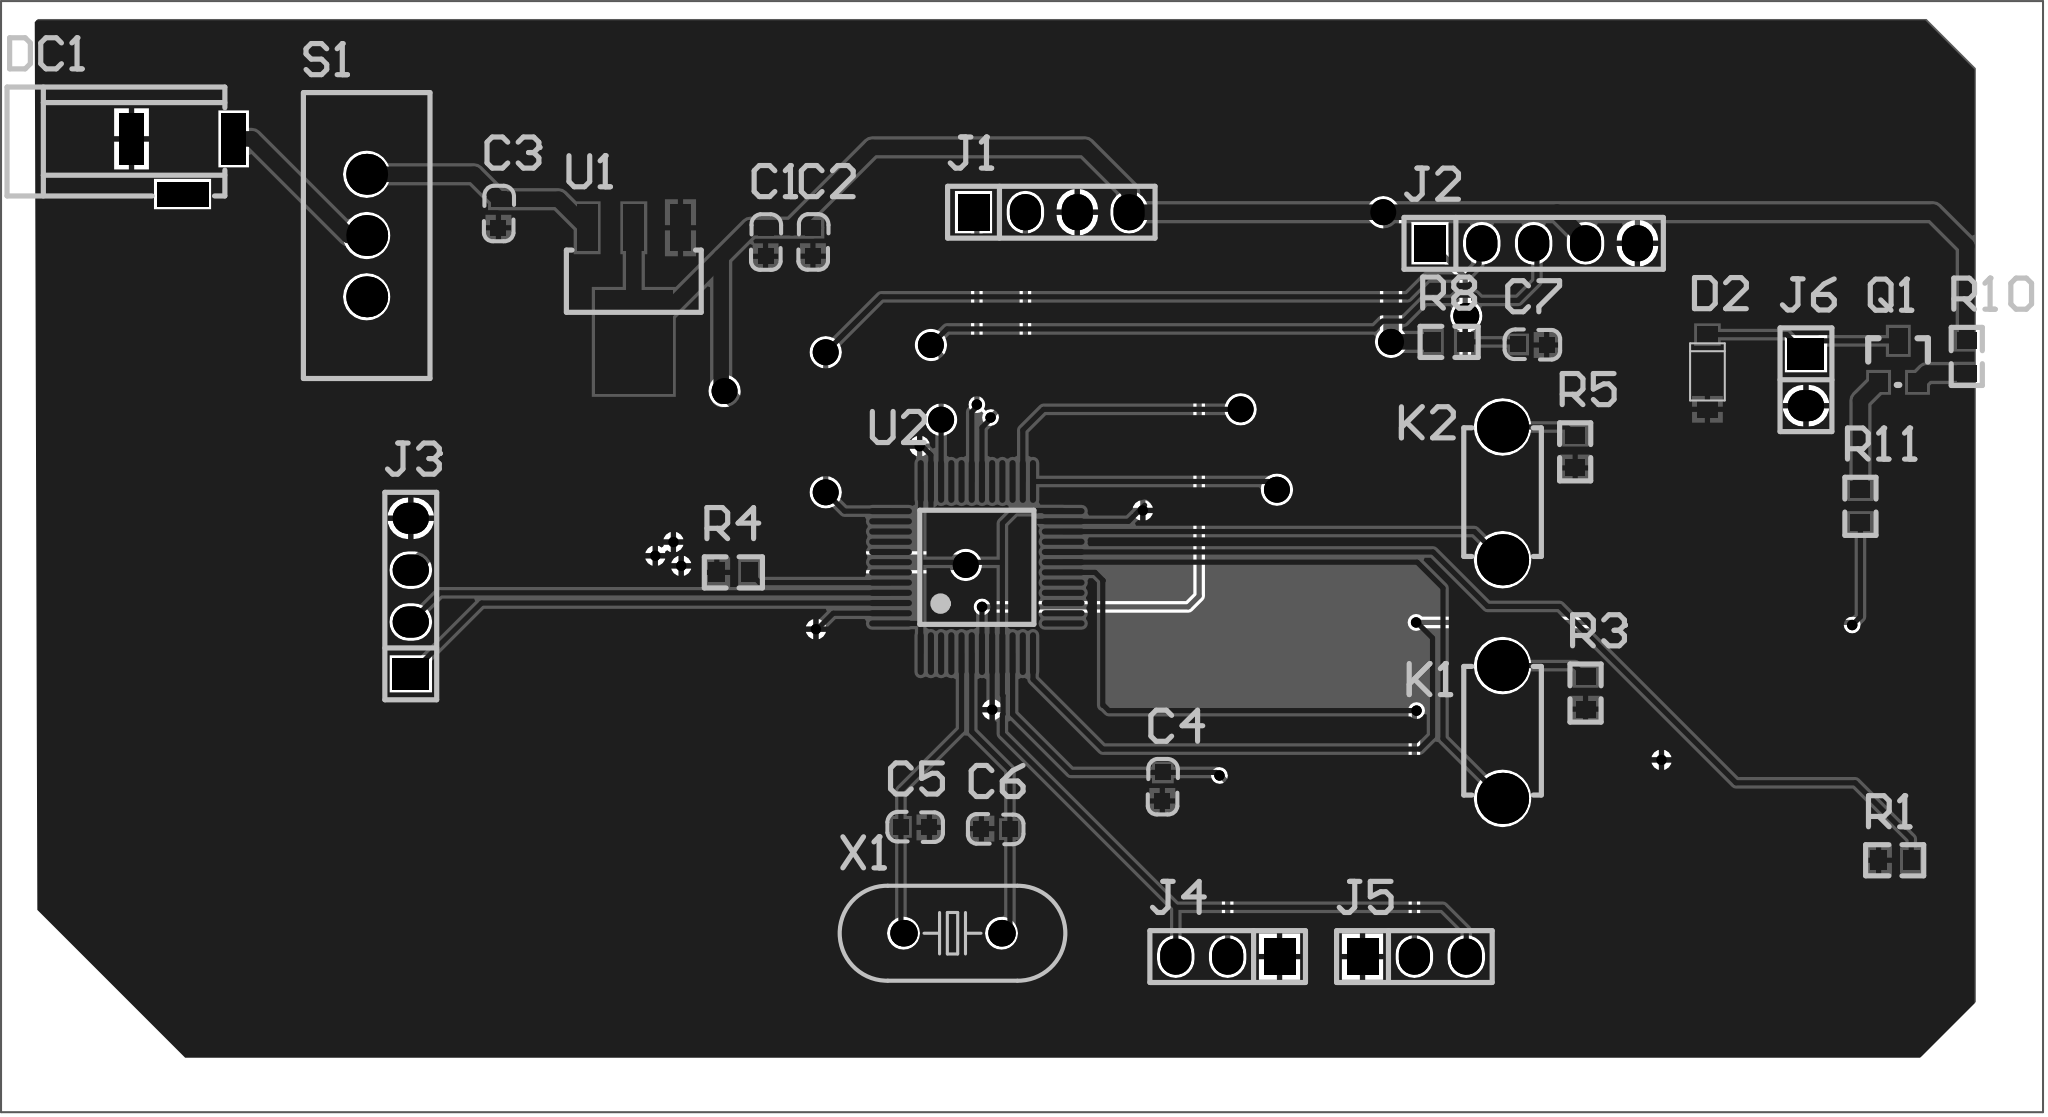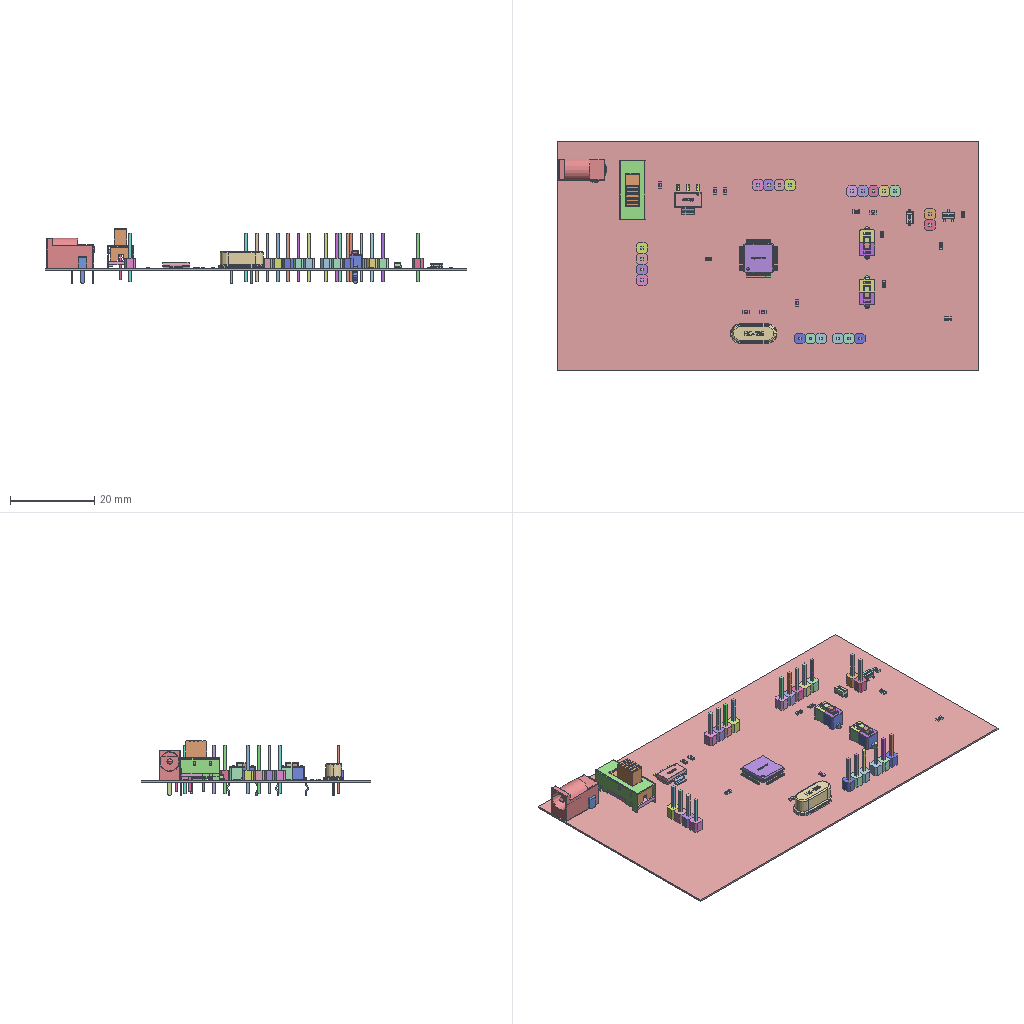Circuit board layout | Altium Designer | box 100 x 54.4 x 13.1 mm
Layer stack:
# Altium Designer layer stack of  (unit mm; dielectric type: 0 none, 1 core, 2 prepreg, 3 surface material)
index,name,kind,layer,copper_thickness_mm,dielectric_type,dielectric_thickness_mm,dielectric_material,dielectric_constant
0,Top Paste,other,,,,,,
1,Top Overlay,other,,,,,,
2,Top Solder,dielectric,,,3,0.0102,Solder Resist,3.5
3,Top Layer,copper,Top Layer,0.0356,,,,
4,Dielectric 1,dielectric,,,0,0.32,FR-4,4.8
5,Bottom Layer,copper,Bottom Layer,0.0356,,,,
6,Bottom Solder,dielectric,,,3,0.0102,Solder Resist,3.5
7,Bottom Overlay,other,,,,,,
8,Bottom Paste,other,,,,,,
# drill layer pairs: low layer,high layer
drill_pair,Top Layer,Bottom Layer
Part placement:
Designator,Comment,Layer,Footprint,Center-X(mm),Center-Y(mm),Rotation
Q1,PNP,TopLayer,SOT-23,92.9,82.347,0
J6,Pin HDR1X2,TopLayer,Pin_HDR1X2/2.54mm-S,88.392,81.458,0
J5,Pin HDR1X3,TopLayer,Pin_HDR1X3/2.54mm-S,69.215,53.213,90
J4,Pin HDR1X3,TopLayer,Pin_HDR1X3/2.54mm-S,60.071,53.213,270
D2,DIODE,TopLayer,SOD-123,83.566,81.839,90
X1,XTAL-2P,TopLayer,OSC_HC-49S,46.596,54.356,360
U2,STM32F103C8T6,TopLayer,LQFP48_7X7,47.788,72.262,0
U1,AMS1117,TopLayer,SOT223,30.988,86.106,180
S1,SS-12D10,TopLayer,SS-12D10,17.907,88.519,270
R11,470,TopLayer,0603R,91.059,75.273,90
R10,470,TopLayer,0603R,96.266,82.588,270
R8,10K,TopLayer,0603R,70.904,83.312,180
R5,10K,TopLayer,0603R,77.089,77.94,90
R4,10K,TopLayer,0603R,35.852,72.025,180
R3,10K,TopLayer,0603R,77.597,66.129,90
R1,10K,TopLayer,0603R,92.748,57.929,0
K2,KEY,TopLayer,DIP-3X6X4.3,73.533,75.894,90
K1,KEY,TopLayer,DIP-3X6X4.3,73.533,64.21,90
J3,Pin HDR1X4,TopLayer,Pin_HDR1X4/2.54mm-S,20.066,70.866,180
J2,Pin HDR1X5,TopLayer,Pin_HDR1X5/2.54mm-S,75.057,88.138,90
J1,Pin HDR1X4,TopLayer,Pin_HDR1X4/2.54mm-S,51.435,89.662,90
DC1,DC_Socket,TopLayer,DC-002,8.89,91.901,180
C7,0.1uF,TopLayer,0603C,74.993,83.172,180
C6,20pF,TopLayer,0603C,48.71,59.465,0
C5,20pF,TopLayer,0603C,44.767,59.55,180
C4,0.1uF,TopLayer,0603C,56.883,61.532,90
C3,10uF,TopLayer,0603C,24.371,89.599,90
C2,0.1uF,TopLayer,0603C,39.773,88.207,90
C1,10uF,TopLayer,0603C,37.452,88.201,90
Pad and via stacks:
# Altium Designer via and pad stacks of  (unit mm). Each distinct definition once, with the count of objects using it.
# via: kind,start_layer,end_layer,hole_mm,diameter_mm,mode(0 simple;1 top-mid-bottom;2 full stack),diameter_per_layer,count,example_net
# pad: kind,layer,hole_mm,hole_type(0 round;1 square;2 slot),plating,top_size,top_shape(1 round;2 rect;3 octagon;9 rounded rect),mid_size,bottom_size,mode,footprint,size_per_layer,count,example
pad,Top Layer,0,0,plated,0.9144x0.9144,2,0.9144x0.9144,0.9144x0.9144,0,SOT-23,,2,Q1.B
pad,Top Layer,0,0,plated,0.9144x1.27,2,0.9144x1.27,0.9144x1.27,0,SOT-23,,1,Q1.C
pad,Top Layer,0,0,plated,1x0.8,2,1x0.8,1x0.8,0,SOD-123,,2,D2.A
pad,Top Layer,0,0,plated,1.016x2.286,2,1.016x2.286,1.016x2.286,0,SOT223,,3,U1.3
pad,Top Layer,0,0,plated,3.81x5.08,2,3.81x5.08,3.81x5.08,0,SOT223,,1,U1.2
pad,Top Layer,0,0,plated,0.3x2.1,1,0.3x2.1,0.3x2.1,0,LQFP48 7X7,,48,U2.48
pad,Top Layer,0,0,plated,0.762x0.762,2,0.762x0.762,0.762x0.762,0,0603C,,14,C2.2
pad,Top Layer,0,0,plated,0.8x0.965,2,0.8x0.965,0.8x0.965,0,0603R,,14,R1.2
pad,Multi-Layer,0.8128,0,plated,1.524x1.778,1,1.524x1.778,1.524x1.778,0,Pin HDR1X5/2.54mm-S,,4,J2.5
pad,Multi-Layer,0.8128,0,plated,1.524x1.778,2,1.524x1.778,1.524x1.778,0,Pin HDR1X5/2.54mm-S,,1,J2.1
pad,Multi-Layer,0.8128,0,plated,1.524x1.778,1,1.524x1.778,1.524x1.778,0,Pin HDR1X3/2.54mm-S,,4,J5.3
pad,Multi-Layer,0.8128,0,plated,1.524x1.778,2,1.524x1.778,1.524x1.778,0,Pin HDR1X3/2.54mm-S,,2,J5.1
pad,Multi-Layer,0.8128,0,plated,1.524x1.778,1,1.524x1.778,1.524x1.778,0,Pin HDR1X2/2.54mm-S,,1,J6.2
pad,Multi-Layer,0.8128,0,plated,1.524x1.778,2,1.524x1.778,1.524x1.778,0,Pin HDR1X2/2.54mm-S,,1,J6.1
pad,Multi-Layer,1.2,0,plated,2.5x2.5,1,2.5x2.5,2.5x2.5,0,DIP-3X6X4.3,,4,K1.1
pad,Multi-Layer,0.6,2,plated,2.5x1.2,2,2.5x1.2,2.5x1.2,0,DC-002,,3,DC1.3
pad,Multi-Layer,1.2,0,plated,2x2,1,2x2,2x2,0,SS-12D10,,3,S1.2
pad,Multi-Layer,0.8128,0,plated,1.524x1.778,1,1.524x1.778,1.524x1.778,0,Pin HDR1X4/2.54mm-S,,6,J3.4
pad,Multi-Layer,0.8128,0,plated,1.524x1.778,2,1.524x1.778,1.524x1.778,0,Pin HDR1X4/2.54mm-S,,2,J3.1
pad,Multi-Layer,0.6,0,plated,1.3x1.3,1,1.3x1.3,1.3x1.3,0,OSC HC-49S,,2,X1.1
via,Top Layer,Bottom Layer,0.254,0.508,0,,15,pwm
via,Top Layer,Bottom Layer,0.7112,1.27,0,,11,VCC
Copper pours:
name,layer,net,type(0 solid;1 hatched;2 none)
Top Layer-GND,Top Layer,GND,0
Bottom Layer-GND,Bottom Layer,GND,0
Design rules, without the lines most boards share:
# Altium Designer design rules of  (exported by Altium Designer, unit mm)
# columns: name | kind | enabled | priority | scope1 | scope2 | descriptor | typed fields (field=value)
HoleToHoleClearance | 52 | enabled | 1 | All | All | Hole To Hole Clearance (Gap=10mil) (All),(All) | gap=0.254
DiffPairsRouting | 51 | enabled | 1 | All | All | Differential Pairs Uncoupled Length using the Gap Constraints (Min=10mil) (Max=10mil) (Prefered=10mil)  and Width Constraints (Min=15mil) (Max=15mil) (Prefered=15mil) (All) |
SolderMaskExpansion | 13 | enabled | 1 | All | All | Solder Mask Expansion (Expansion =4mil) (All) | expansion=0.1016
PasteMaskExpansion | 14 | enabled | 1 | All | All | Paste Mask Expansion (Expansion =0mil) (All) | expansion=0
RoutingVias | 11 | enabled | 1 | All | All | Routing Via (MinHoleWidth=10mil) (MaxHoleWidth=10mil) (PreferredHoleWidth=10mil) (MinWidth=20mil) (MaxWidth=50mil) (PreferedWidth=20mil) (All) | via_min_hole=0.254 via_max_hole=0.254 via_preferred_diameter=0.508 via_preferred_hole=0.254
Width | 2 | enabled | 1 | All | All | Width Constraint (Min=10mil) (Max=50mil) (Preferred=10mil) (All) |
PolygonConnect | 20 | enabled | 1 | All | All | Polygon Connect Rule(Relief Connect )(Conductor Width=10mil) (Relief Angle=90 Angle) (Entries=4) (Air Gap Width=10mil) (All),(All) | connect_style(0=relief,1=direct,2=none)=0 relief_conductor_width=0.254 relief_entries=4
PlaneConnect | 6 | enabled | 1 | All | All | Power Plane Connect Rule(Relief Connect )(Expansion=20mil) (Conductor Width=10mil) (Air Gap=10mil) (Entries=4) (All) | relief_conductor_width=0.254 relief_entries=4 relief_expansion=0.508
Clearance | 0 | enabled | 1 | All | All | Clearance Constraint (Gap=6mil) (All),(All) | gap=0.1524
Classes set for this board:
# Altium Designer classes of  (member kind: 0 net, 1 component, 2 from-to, 3 pad, 4 layer, 5 differential pair, 6 design channel, 7 polygon, 8 structure, 9 xSignal)
# columns: class name | member kind | superclass | members
Sheet1 | 1 | no | C1; C2; C3; C4; C5; C6; C7; DC1; J1; J2; J3; K1; K2; R1; R3; R4; R5; R8; R10; R11; S1; U1; U2; X1; J4; J5; J6; Q1; D2;